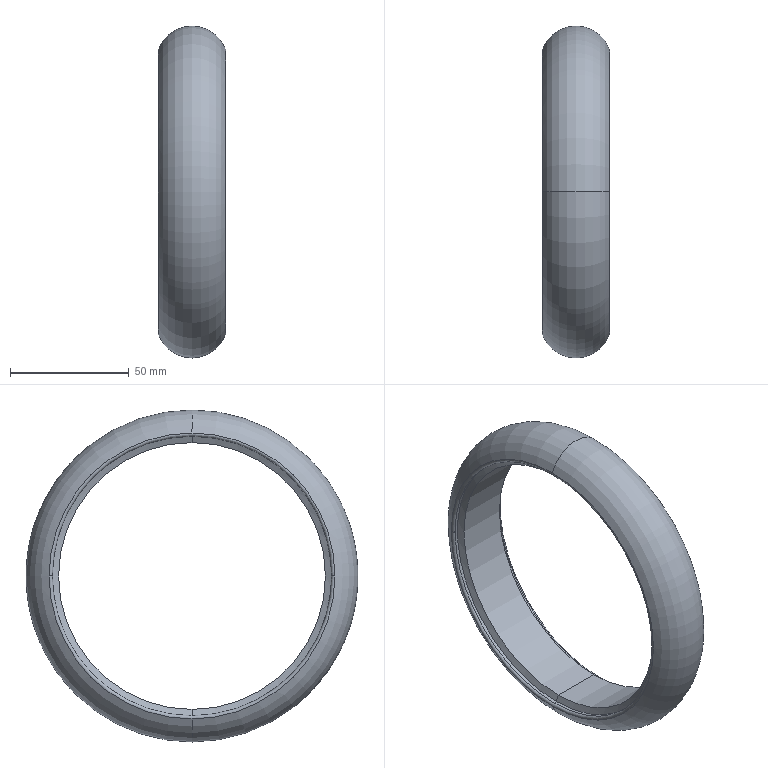Part | SolidWorks | features BaseBody 1 | 1 solid | 16 faces | box 28.26 x 139.7 x 139.7 mm | volume 115471 mm3 | torus 6 | cylinder 6 | cone 4 | commonest cylinder face diameters 117.58 x4 112.289 x2
STEP:
#1=CARTESIAN_POINT('',(238.404,144.664,-523.955));
#2=VERTEX_POINT('',#1);
#3=CARTESIAN_POINT('',(238.404,84.519,-463.81));
#4=VERTEX_POINT('',#3);
#5=CARTESIAN_POINT('',(238.404,84.519,-523.955));
#6=DIRECTION('',(1.,0.,0.));
#7=DIRECTION('',(0.,0.,-1.));
#8=AXIS2_PLACEMENT_3D('',#5,#6,#7);
#9=CIRCLE('',#8,60.145);
#10=EDGE_CURVE('',#2,#4,#9,.T.);
#11=ORIENTED_EDGE('',*,*,#10,.T.);
#12=CARTESIAN_POINT('',(266.534,84.519,-463.81));
#13=VERTEX_POINT('',#12);
#14=CARTESIAN_POINT('',(252.469,84.519,-469.149));
#15=DIRECTION('',(0.,1.,0.));
#16=DIRECTION('',(0.,0.,1.));
#17=AXIS2_PLACEMENT_3D('',#14,#15,#16);
#18=CIRCLE('',#17,15.045);
#19=EDGE_CURVE('',#4,#13,#18,.T.);
#20=ORIENTED_EDGE('',*,*,#19,.T.);
#21=CARTESIAN_POINT('',(266.534,84.519,-584.1));
#22=VERTEX_POINT('',#21);
#23=CARTESIAN_POINT('',(266.534,84.519,-523.955));
#24=DIRECTION('',(-1.,0.,0.));
#25=DIRECTION('',(0.,0.,1.));
#26=AXIS2_PLACEMENT_3D('',#23,#24,#25);
#27=CIRCLE('',#26,60.145);
#28=EDGE_CURVE('',#13,#22,#27,.T.);
#29=ORIENTED_EDGE('',*,*,#28,.T.);
#30=CARTESIAN_POINT('',(238.404,84.519,-584.1));
#31=VERTEX_POINT('',#30);
#32=CARTESIAN_POINT('',(252.469,84.519,-578.76));
#33=DIRECTION('',(0.,-1.,0.));
#34=DIRECTION('',(0.,0.,-1.));
#35=AXIS2_PLACEMENT_3D('',#32,#33,#34);
#36=CIRCLE('',#35,15.045);
#37=EDGE_CURVE('',#31,#22,#36,.T.);
#38=ORIENTED_EDGE('',*,*,#37,.F.);
#39=CARTESIAN_POINT('',(238.404,84.519,-523.955));
#40=DIRECTION('',(1.,0.,0.));
#41=DIRECTION('',(0.,0.,-1.));
#42=AXIS2_PLACEMENT_3D('',#39,#40,#41);
#43=CIRCLE('',#42,60.145);
#44=EDGE_CURVE('',#31,#2,#43,.T.);
#45=ORIENTED_EDGE('',*,*,#44,.T.);
#46=EDGE_LOOP('',(#11,#20,#29,#38,#45));
#47=FACE_OUTER_BOUND('',#46,.T.);
#48=CARTESIAN_POINT('',(252.469,84.519,-523.955));
#49=DIRECTION('',(1.,0.,0.));
#50=DIRECTION('',(0.,0.,-1.));
#51=AXIS2_PLACEMENT_3D('',#48,#49,#50);
#52=TOROIDAL_SURFACE('',#51,54.805,15.045);
#53=ADVANCED_FACE('',(#47),#52,.T.);
#54=ORIENTED_EDGE('',*,*,#10,.F.);
#55=CARTESIAN_POINT('',(239.338,143.309,-523.955));
#56=VERTEX_POINT('',#55);
#57=CARTESIAN_POINT('',(239.338,144.309,-523.955));
#58=DIRECTION('',(0.,0.,1.));
#59=DIRECTION('',(0.,-1.,0.));
#60=AXIS2_PLACEMENT_3D('',#57,#58,#59);
#61=CIRCLE('',#60,1.);
#62=EDGE_CURVE('',#2,#56,#61,.T.);
#63=ORIENTED_EDGE('',*,*,#62,.T.);
#64=CARTESIAN_POINT('',(239.338,84.519,-465.164));
#65=VERTEX_POINT('',#64);
#66=CARTESIAN_POINT('',(239.338,84.519,-523.955));
#67=DIRECTION('',(1.,0.,0.));
#68=DIRECTION('',(0.,1.,0.));
#69=AXIS2_PLACEMENT_3D('',#66,#67,#68);
#70=CIRCLE('',#69,58.79);
#71=EDGE_CURVE('',#56,#65,#70,.T.);
#72=ORIENTED_EDGE('',*,*,#71,.T.);
#73=CARTESIAN_POINT('',(239.338,25.729,-523.955));
#74=VERTEX_POINT('',#73);
#75=CARTESIAN_POINT('',(239.338,84.519,-523.955));
#76=DIRECTION('',(1.,0.,0.));
#77=DIRECTION('',(0.,1.,0.));
#78=AXIS2_PLACEMENT_3D('',#75,#76,#77);
#79=CIRCLE('',#78,58.79);
#80=EDGE_CURVE('',#65,#74,#79,.T.);
#81=ORIENTED_EDGE('',*,*,#80,.T.);
#82=CARTESIAN_POINT('',(238.404,24.374,-523.955));
#83=VERTEX_POINT('',#82);
#84=CARTESIAN_POINT('',(239.338,24.729,-523.955));
#85=DIRECTION('',(0.,0.,-1.));
#86=DIRECTION('',(-1.,0.,0.));
#87=AXIS2_PLACEMENT_3D('',#84,#85,#86);
#88=CIRCLE('',#87,1.);
#89=EDGE_CURVE('',#83,#74,#88,.T.);
#90=ORIENTED_EDGE('',*,*,#89,.F.);
#91=CARTESIAN_POINT('',(238.404,84.519,-523.955));
#92=DIRECTION('',(1.,0.,0.));
#93=DIRECTION('',(0.,0.,-1.));
#94=AXIS2_PLACEMENT_3D('',#91,#92,#93);
#95=CIRCLE('',#94,60.145);
#96=EDGE_CURVE('',#4,#83,#95,.T.);
#97=ORIENTED_EDGE('',*,*,#96,.F.);
#98=EDGE_LOOP('',(#54,#63,#72,#81,#90,#97));
#99=FACE_OUTER_BOUND('',#98,.T.);
#100=CARTESIAN_POINT('',(239.338,84.519,-523.955));
#101=DIRECTION('',(-1.,0.,0.));
#102=DIRECTION('',(0.,-1.,0.));
#103=AXIS2_PLACEMENT_3D('',#100,#101,#102);
#104=TOROIDAL_SURFACE('',#103,59.79,1.);
#105=ADVANCED_FACE('',(#99),#104,.T.);
#106=ORIENTED_EDGE('',*,*,#80,.F.);
#107=CARTESIAN_POINT('',(240.679,84.519,-465.164));
#108=VERTEX_POINT('',#107);
#109=CARTESIAN_POINT('',(237.951,84.519,-465.164));
#110=DIRECTION('',(1.,0.,0.));
#111=VECTOR('',#110,1000.);
#112=LINE('',#109,#111);
#113=EDGE_CURVE('',#65,#108,#112,.T.);
#114=ORIENTED_EDGE('',*,*,#113,.T.);
#115=CARTESIAN_POINT('',(240.679,84.519,-582.745));
#116=VERTEX_POINT('',#115);
#117=CARTESIAN_POINT('',(240.679,84.519,-523.955));
#118=DIRECTION('',(-1.,0.,0.));
#119=DIRECTION('',(0.,0.,-1.));
#120=AXIS2_PLACEMENT_3D('',#117,#118,#119);
#121=CIRCLE('',#120,58.79);
#122=EDGE_CURVE('',#116,#108,#121,.T.);
#123=ORIENTED_EDGE('',*,*,#122,.F.);
#124=CARTESIAN_POINT('',(239.338,84.519,-582.745));
#125=VERTEX_POINT('',#124);
#126=CARTESIAN_POINT('',(237.951,84.519,-582.745));
#127=DIRECTION('',(1.,0.,0.));
#128=VECTOR('',#127,1000.);
#129=LINE('',#126,#128);
#130=EDGE_CURVE('',#125,#116,#129,.T.);
#131=ORIENTED_EDGE('',*,*,#130,.F.);
#132=CARTESIAN_POINT('',(239.338,84.519,-523.955));
#133=DIRECTION('',(1.,0.,0.));
#134=DIRECTION('',(0.,1.,0.));
#135=AXIS2_PLACEMENT_3D('',#132,#133,#134);
#136=CIRCLE('',#135,58.79);
#137=EDGE_CURVE('',#74,#125,#136,.T.);
#138=ORIENTED_EDGE('',*,*,#137,.F.);
#139=EDGE_LOOP('',(#106,#114,#123,#131,#138));
#140=FACE_OUTER_BOUND('',#139,.T.);
#141=CARTESIAN_POINT('',(237.951,84.519,-523.955));
#142=DIRECTION('',(1.,0.,0.));
#143=DIRECTION('',(0.,0.,-1.));
#144=AXIS2_PLACEMENT_3D('',#141,#142,#143);
#145=CYLINDRICAL_SURFACE('',#144,58.79);
#146=ADVANCED_FACE('',(#140),#145,.F.);
#147=ORIENTED_EDGE('',*,*,#28,.F.);
#148=CARTESIAN_POINT('',(265.599,84.519,-465.164));
#149=VERTEX_POINT('',#148);
#150=CARTESIAN_POINT('',(265.599,84.519,-464.164));
#151=DIRECTION('',(0.,1.,0.));
#152=DIRECTION('',(0.,0.,1.));
#153=AXIS2_PLACEMENT_3D('',#150,#151,#152);
#154=CIRCLE('',#153,1.);
#155=EDGE_CURVE('',#13,#149,#154,.T.);
#156=ORIENTED_EDGE('',*,*,#155,.T.);
#157=CARTESIAN_POINT('',(265.599,84.519,-582.745));
#158=VERTEX_POINT('',#157);
#159=CARTESIAN_POINT('',(265.599,84.519,-523.955));
#160=DIRECTION('',(-1.,0.,0.));
#161=DIRECTION('',(0.,0.,1.));
#162=AXIS2_PLACEMENT_3D('',#159,#160,#161);
#163=CIRCLE('',#162,58.79);
#164=EDGE_CURVE('',#149,#158,#163,.T.);
#165=ORIENTED_EDGE('',*,*,#164,.T.);
#166=CARTESIAN_POINT('',(265.599,84.519,-583.745));
#167=DIRECTION('',(0.,-1.,0.));
#168=DIRECTION('',(0.,0.,-1.));
#169=AXIS2_PLACEMENT_3D('',#166,#167,#168);
#170=CIRCLE('',#169,1.);
#171=EDGE_CURVE('',#22,#158,#170,.T.);
#172=ORIENTED_EDGE('',*,*,#171,.F.);
#173=EDGE_LOOP('',(#147,#156,#165,#172));
#174=FACE_OUTER_BOUND('',#173,.T.);
#175=CARTESIAN_POINT('',(265.599,84.519,-523.955));
#176=DIRECTION('',(1.,0.,0.));
#177=DIRECTION('',(0.,0.,-1.));
#178=AXIS2_PLACEMENT_3D('',#175,#176,#177);
#179=TOROIDAL_SURFACE('',#178,59.79,1.);
#180=ADVANCED_FACE('',(#174),#179,.T.);
#181=CARTESIAN_POINT('',(241.955,84.519,-580.099));
#182=VERTEX_POINT('',#181);
#183=CARTESIAN_POINT('',(241.955,84.519,-467.81));
#184=VERTEX_POINT('',#183);
#185=CARTESIAN_POINT('',(241.955,84.519,-523.955));
#186=DIRECTION('',(-1.,0.,0.));
#187=DIRECTION('',(0.,-1.,0.));
#188=AXIS2_PLACEMENT_3D('',#185,#186,#187);
#189=CIRCLE('',#188,56.145);
#190=EDGE_CURVE('',#182,#184,#189,.T.);
#191=ORIENTED_EDGE('',*,*,#190,.F.);
#192=CARTESIAN_POINT('',(240.679,84.519,-582.745));
#193=DIRECTION('',(-0.4346,0.,-0.9006));
#194=VECTOR('',#193,1000.);
#195=LINE('',#192,#194);
#196=EDGE_CURVE('',#182,#116,#195,.T.);
#197=ORIENTED_EDGE('',*,*,#196,.T.);
#198=ORIENTED_EDGE('',*,*,#122,.T.);
#199=CARTESIAN_POINT('',(240.679,84.519,-465.164));
#200=DIRECTION('',(-0.4346,0.,0.9006));
#201=VECTOR('',#200,1000.);
#202=LINE('',#199,#201);
#203=EDGE_CURVE('',#184,#108,#202,.T.);
#204=ORIENTED_EDGE('',*,*,#203,.F.);
#205=EDGE_LOOP('',(#191,#197,#198,#204));
#206=FACE_OUTER_BOUND('',#205,.T.);
#207=CARTESIAN_POINT('',(240.679,84.519,-523.955));
#208=DIRECTION('',(-1.,0.,0.));
#209=DIRECTION('',(0.,0.,1.));
#210=AXIS2_PLACEMENT_3D('',#207,#208,#209);
#211=CONICAL_SURFACE('',#210,58.79,1.121);
#212=ADVANCED_FACE('',(#206),#211,.F.);
#213=CARTESIAN_POINT('',(264.353,84.519,-465.164));
#214=VERTEX_POINT('',#213);
#215=CARTESIAN_POINT('',(264.353,84.519,-582.745));
#216=VERTEX_POINT('',#215);
#217=CARTESIAN_POINT('',(264.353,84.519,-523.955));
#218=DIRECTION('',(1.,0.,0.));
#219=DIRECTION('',(0.,0.,-1.));
#220=AXIS2_PLACEMENT_3D('',#217,#218,#219);
#221=CIRCLE('',#220,58.79);
#222=EDGE_CURVE('',#214,#216,#221,.T.);
#223=ORIENTED_EDGE('',*,*,#222,.F.);
#224=CARTESIAN_POINT('',(237.951,84.519,-465.164));
#225=DIRECTION('',(1.,0.,0.));
#226=VECTOR('',#225,1000.);
#227=LINE('',#224,#226);
#228=EDGE_CURVE('',#214,#149,#227,.T.);
#229=ORIENTED_EDGE('',*,*,#228,.T.);
#230=CARTESIAN_POINT('',(265.599,84.519,-523.955));
#231=DIRECTION('',(-1.,0.,0.));
#232=DIRECTION('',(0.,0.,1.));
#233=AXIS2_PLACEMENT_3D('',#230,#231,#232);
#234=CIRCLE('',#233,58.79);
#235=EDGE_CURVE('',#158,#149,#234,.T.);
#236=ORIENTED_EDGE('',*,*,#235,.F.);
#237=CARTESIAN_POINT('',(237.951,84.519,-582.745));
#238=DIRECTION('',(1.,0.,0.));
#239=VECTOR('',#238,1000.);
#240=LINE('',#237,#239);
#241=EDGE_CURVE('',#216,#158,#240,.T.);
#242=ORIENTED_EDGE('',*,*,#241,.F.);
#243=EDGE_LOOP('',(#223,#229,#236,#242));
#244=FACE_OUTER_BOUND('',#243,.T.);
#245=CARTESIAN_POINT('',(237.951,84.519,-523.955));
#246=DIRECTION('',(1.,0.,0.));
#247=DIRECTION('',(0.,0.,-1.));
#248=AXIS2_PLACEMENT_3D('',#245,#246,#247);
#249=CYLINDRICAL_SURFACE('',#248,58.79);
#250=ADVANCED_FACE('',(#244),#249,.F.);
#251=CARTESIAN_POINT('',(263.039,84.519,-580.099));
#252=VERTEX_POINT('',#251);
#253=CARTESIAN_POINT('',(263.039,84.519,-467.81));
#254=VERTEX_POINT('',#253);
#255=CARTESIAN_POINT('',(263.039,84.519,-523.955));
#256=DIRECTION('',(-1.,0.,0.));
#257=DIRECTION('',(0.,0.,1.));
#258=AXIS2_PLACEMENT_3D('',#255,#256,#257);
#259=CIRCLE('',#258,56.145);
#260=EDGE_CURVE('',#252,#254,#259,.T.);
#261=ORIENTED_EDGE('',*,*,#260,.F.);
#262=CARTESIAN_POINT('',(237.2,84.519,-580.099));
#263=DIRECTION('',(-1.,0.,0.));
#264=VECTOR('',#263,1000.);
#265=LINE('',#262,#264);
#266=EDGE_CURVE('',#252,#182,#265,.T.);
#267=ORIENTED_EDGE('',*,*,#266,.T.);
#268=ORIENTED_EDGE('',*,*,#190,.T.);
#269=CARTESIAN_POINT('',(237.2,84.519,-467.81));
#270=DIRECTION('',(-1.,0.,0.));
#271=VECTOR('',#270,1000.);
#272=LINE('',#269,#271);
#273=EDGE_CURVE('',#254,#184,#272,.T.);
#274=ORIENTED_EDGE('',*,*,#273,.F.);
#275=EDGE_LOOP('',(#261,#267,#268,#274));
#276=FACE_OUTER_BOUND('',#275,.T.);
#277=CARTESIAN_POINT('',(237.2,84.519,-523.955));
#278=DIRECTION('',(-1.,0.,0.));
#279=DIRECTION('',(0.,0.,1.));
#280=AXIS2_PLACEMENT_3D('',#277,#278,#279);
#281=CYLINDRICAL_SURFACE('',#280,56.145);
#282=ADVANCED_FACE('',(#276),#281,.F.);
#283=ORIENTED_EDGE('',*,*,#260,.T.);
#284=CARTESIAN_POINT('',(264.353,84.519,-465.164));
#285=DIRECTION('',(0.4449,0.,0.8956));
#286=VECTOR('',#285,1000.);
#287=LINE('',#284,#286);
#288=EDGE_CURVE('',#254,#214,#287,.T.);
#289=ORIENTED_EDGE('',*,*,#288,.T.);
#290=ORIENTED_EDGE('',*,*,#222,.T.);
#291=CARTESIAN_POINT('',(264.353,84.519,-582.745));
#292=DIRECTION('',(0.4449,0.,-0.8956));
#293=VECTOR('',#292,1000.);
#294=LINE('',#291,#293);
#295=EDGE_CURVE('',#252,#216,#294,.T.);
#296=ORIENTED_EDGE('',*,*,#295,.F.);
#297=EDGE_LOOP('',(#283,#289,#290,#296));
#298=FACE_OUTER_BOUND('',#297,.T.);
#299=CARTESIAN_POINT('',(264.353,84.519,-523.955));
#300=DIRECTION('',(1.,0.,0.));
#301=DIRECTION('',(0.,0.,-1.));
#302=AXIS2_PLACEMENT_3D('',#299,#300,#301);
#303=CONICAL_SURFACE('',#302,58.79,1.11);
#304=ADVANCED_FACE('',(#298),#303,.F.);
#305=ORIENTED_EDGE('',*,*,#19,.F.);
#306=ORIENTED_EDGE('',*,*,#96,.T.);
#307=CARTESIAN_POINT('',(238.404,84.519,-523.955));
#308=DIRECTION('',(1.,0.,0.));
#309=DIRECTION('',(0.,0.,-1.));
#310=AXIS2_PLACEMENT_3D('',#307,#308,#309);
#311=CIRCLE('',#310,60.145);
#312=EDGE_CURVE('',#83,#31,#311,.T.);
#313=ORIENTED_EDGE('',*,*,#312,.T.);
#314=ORIENTED_EDGE('',*,*,#37,.T.);
#315=CARTESIAN_POINT('',(266.534,84.519,-523.955));
#316=DIRECTION('',(-1.,0.,0.));
#317=DIRECTION('',(0.,0.,1.));
#318=AXIS2_PLACEMENT_3D('',#315,#316,#317);
#319=CIRCLE('',#318,60.145);
#320=EDGE_CURVE('',#22,#13,#319,.T.);
#321=ORIENTED_EDGE('',*,*,#320,.T.);
#322=EDGE_LOOP('',(#305,#306,#313,#314,#321));
#323=FACE_OUTER_BOUND('',#322,.T.);
#324=CARTESIAN_POINT('',(252.469,84.519,-523.955));
#325=DIRECTION('',(1.,0.,0.));
#326=DIRECTION('',(0.,0.,-1.));
#327=AXIS2_PLACEMENT_3D('',#324,#325,#326);
#328=TOROIDAL_SURFACE('',#327,54.805,15.045);
#329=ADVANCED_FACE('',(#323),#328,.T.);
#330=ORIENTED_EDGE('',*,*,#62,.F.);
#331=ORIENTED_EDGE('',*,*,#44,.F.);
#332=ORIENTED_EDGE('',*,*,#312,.F.);
#333=ORIENTED_EDGE('',*,*,#89,.T.);
#334=ORIENTED_EDGE('',*,*,#137,.T.);
#335=CARTESIAN_POINT('',(239.338,84.519,-523.955));
#336=DIRECTION('',(1.,0.,0.));
#337=DIRECTION('',(0.,1.,0.));
#338=AXIS2_PLACEMENT_3D('',#335,#336,#337);
#339=CIRCLE('',#338,58.79);
#340=EDGE_CURVE('',#125,#56,#339,.T.);
#341=ORIENTED_EDGE('',*,*,#340,.T.);
#342=EDGE_LOOP('',(#330,#331,#332,#333,#334,#341));
#343=FACE_OUTER_BOUND('',#342,.T.);
#344=CARTESIAN_POINT('',(239.338,84.519,-523.955));
#345=DIRECTION('',(-1.,0.,0.));
#346=DIRECTION('',(0.,-1.,0.));
#347=AXIS2_PLACEMENT_3D('',#344,#345,#346);
#348=TOROIDAL_SURFACE('',#347,59.79,1.);
#349=ADVANCED_FACE('',(#343),#348,.T.);
#350=ORIENTED_EDGE('',*,*,#113,.F.);
#351=ORIENTED_EDGE('',*,*,#71,.F.);
#352=ORIENTED_EDGE('',*,*,#340,.F.);
#353=ORIENTED_EDGE('',*,*,#130,.T.);
#354=CARTESIAN_POINT('',(240.679,84.519,-523.955));
#355=DIRECTION('',(-1.,0.,0.));
#356=DIRECTION('',(0.,0.,-1.));
#357=AXIS2_PLACEMENT_3D('',#354,#355,#356);
#358=CIRCLE('',#357,58.79);
#359=EDGE_CURVE('',#108,#116,#358,.T.);
#360=ORIENTED_EDGE('',*,*,#359,.F.);
#361=EDGE_LOOP('',(#350,#351,#352,#353,#360));
#362=FACE_OUTER_BOUND('',#361,.T.);
#363=CARTESIAN_POINT('',(237.951,84.519,-523.955));
#364=DIRECTION('',(1.,0.,0.));
#365=DIRECTION('',(0.,0.,-1.));
#366=AXIS2_PLACEMENT_3D('',#363,#364,#365);
#367=CYLINDRICAL_SURFACE('',#366,58.79);
#368=ADVANCED_FACE('',(#362),#367,.F.);
#369=ORIENTED_EDGE('',*,*,#155,.F.);
#370=ORIENTED_EDGE('',*,*,#320,.F.);
#371=ORIENTED_EDGE('',*,*,#171,.T.);
#372=ORIENTED_EDGE('',*,*,#235,.T.);
#373=EDGE_LOOP('',(#369,#370,#371,#372));
#374=FACE_OUTER_BOUND('',#373,.T.);
#375=CARTESIAN_POINT('',(265.599,84.519,-523.955));
#376=DIRECTION('',(1.,0.,0.));
#377=DIRECTION('',(0.,0.,-1.));
#378=AXIS2_PLACEMENT_3D('',#375,#376,#377);
#379=TOROIDAL_SURFACE('',#378,59.79,1.);
#380=ADVANCED_FACE('',(#374),#379,.T.);
#381=ORIENTED_EDGE('',*,*,#196,.F.);
#382=CARTESIAN_POINT('',(241.955,84.519,-523.955));
#383=DIRECTION('',(-1.,0.,0.));
#384=DIRECTION('',(0.,-1.,0.));
#385=AXIS2_PLACEMENT_3D('',#382,#383,#384);
#386=CIRCLE('',#385,56.145);
#387=EDGE_CURVE('',#184,#182,#386,.T.);
#388=ORIENTED_EDGE('',*,*,#387,.F.);
#389=ORIENTED_EDGE('',*,*,#203,.T.);
#390=ORIENTED_EDGE('',*,*,#359,.T.);
#391=EDGE_LOOP('',(#381,#388,#389,#390));
#392=FACE_OUTER_BOUND('',#391,.T.);
#393=CARTESIAN_POINT('',(240.679,84.519,-523.955));
#394=DIRECTION('',(-1.,0.,0.));
#395=DIRECTION('',(0.,0.,1.));
#396=AXIS2_PLACEMENT_3D('',#393,#394,#395);
#397=CONICAL_SURFACE('',#396,58.79,1.121);
#398=ADVANCED_FACE('',(#392),#397,.F.);
#399=ORIENTED_EDGE('',*,*,#228,.F.);
#400=CARTESIAN_POINT('',(264.353,84.519,-523.955));
#401=DIRECTION('',(1.,0.,0.));
#402=DIRECTION('',(0.,0.,-1.));
#403=AXIS2_PLACEMENT_3D('',#400,#401,#402);
#404=CIRCLE('',#403,58.79);
#405=EDGE_CURVE('',#216,#214,#404,.T.);
#406=ORIENTED_EDGE('',*,*,#405,.F.);
#407=ORIENTED_EDGE('',*,*,#241,.T.);
#408=ORIENTED_EDGE('',*,*,#164,.F.);
#409=EDGE_LOOP('',(#399,#406,#407,#408));
#410=FACE_OUTER_BOUND('',#409,.T.);
#411=CARTESIAN_POINT('',(237.951,84.519,-523.955));
#412=DIRECTION('',(1.,0.,0.));
#413=DIRECTION('',(0.,0.,-1.));
#414=AXIS2_PLACEMENT_3D('',#411,#412,#413);
#415=CYLINDRICAL_SURFACE('',#414,58.79);
#416=ADVANCED_FACE('',(#410),#415,.F.);
#417=ORIENTED_EDGE('',*,*,#266,.F.);
#418=CARTESIAN_POINT('',(263.039,84.519,-523.955));
#419=DIRECTION('',(-1.,0.,0.));
#420=DIRECTION('',(0.,0.,1.));
#421=AXIS2_PLACEMENT_3D('',#418,#419,#420);
#422=CIRCLE('',#421,56.145);
#423=EDGE_CURVE('',#254,#252,#422,.T.);
#424=ORIENTED_EDGE('',*,*,#423,.F.);
#425=ORIENTED_EDGE('',*,*,#273,.T.);
#426=ORIENTED_EDGE('',*,*,#387,.T.);
#427=EDGE_LOOP('',(#417,#424,#425,#426));
#428=FACE_OUTER_BOUND('',#427,.T.);
#429=CARTESIAN_POINT('',(237.2,84.519,-523.955));
#430=DIRECTION('',(-1.,0.,0.));
#431=DIRECTION('',(0.,0.,1.));
#432=AXIS2_PLACEMENT_3D('',#429,#430,#431);
#433=CYLINDRICAL_SURFACE('',#432,56.145);
#434=ADVANCED_FACE('',(#428),#433,.F.);
#435=ORIENTED_EDGE('',*,*,#288,.F.);
#436=ORIENTED_EDGE('',*,*,#423,.T.);
#437=ORIENTED_EDGE('',*,*,#295,.T.);
#438=ORIENTED_EDGE('',*,*,#405,.T.);
#439=EDGE_LOOP('',(#435,#436,#437,#438));
#440=FACE_OUTER_BOUND('',#439,.T.);
#441=CARTESIAN_POINT('',(264.353,84.519,-523.955));
#442=DIRECTION('',(1.,0.,0.));
#443=DIRECTION('',(0.,0.,-1.));
#444=AXIS2_PLACEMENT_3D('',#441,#442,#443);
#445=CONICAL_SURFACE('',#444,58.79,1.11);
#446=ADVANCED_FACE('',(#440),#445,.F.);
#447=CLOSED_SHELL('',(#53,#105,#146,#180,#212,#250,#282,#304,#329,#349,#368,#380,#398,#416,#434,#446));
#448=MANIFOLD_SOLID_BREP('',#447);
#449=CARTESIAN_POINT('',(0.,0.,0.));
#450=DIRECTION('',(0.,0.,1.));
#451=DIRECTION('',(1.,0.,0.));
#452=AXIS2_PLACEMENT_3D('',#449,#450,#451);
#453=(LENGTH_UNIT()NAMED_UNIT(*)SI_UNIT(.MILLI.,.METRE.));
#454=UNCERTAINTY_MEASURE_WITH_UNIT(LENGTH_MEASURE(0.00001),#453,'','');
#455=(NAMED_UNIT(*)PLANE_ANGLE_UNIT()SI_UNIT($,.RADIAN.));
#456=(NAMED_UNIT(*)SI_UNIT($,.STERADIAN.)SOLID_ANGLE_UNIT());
#457=(GEOMETRIC_REPRESENTATION_CONTEXT(3)GLOBAL_UNCERTAINTY_ASSIGNED_CONTEXT((#454))GLOBAL_UNIT_ASSIGNED_CONTEXT((#453,#455,#456))REPRESENTATION_CONTEXT('',''));
#458=ADVANCED_BREP_SHAPE_REPRESENTATION('',(#448,#452),#457);